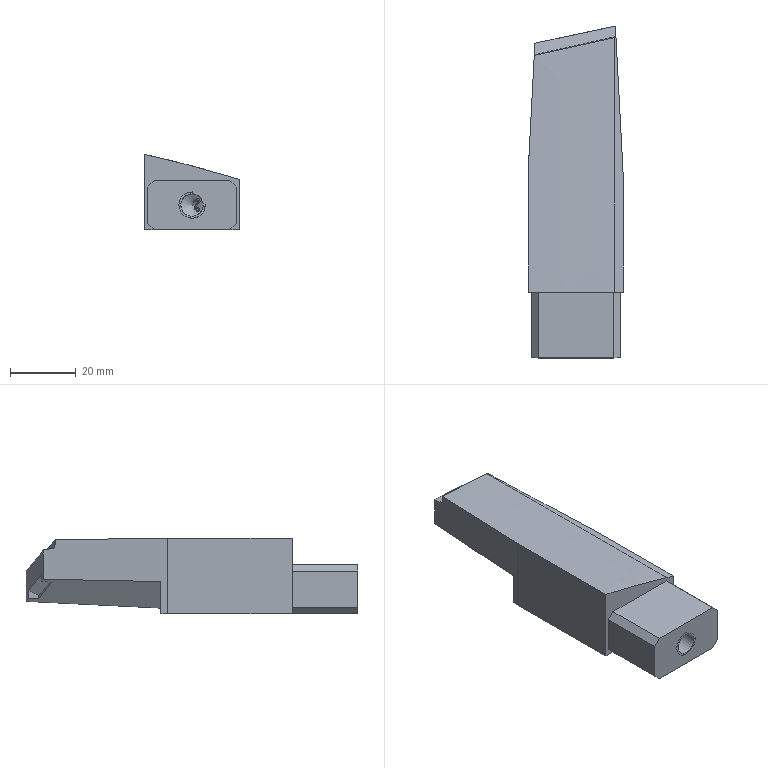Part | STEP file | P011002S004-001 | 1 solid | 60 faces | box 29 x 101.051 x 22.958 mm | volume 42473 mm3 | plane 32 | other 11 | spline 7 | cone 7 | cylinder 3 | commonest cylinder face diameters 6.8 x1 7.973 x1 8 x1